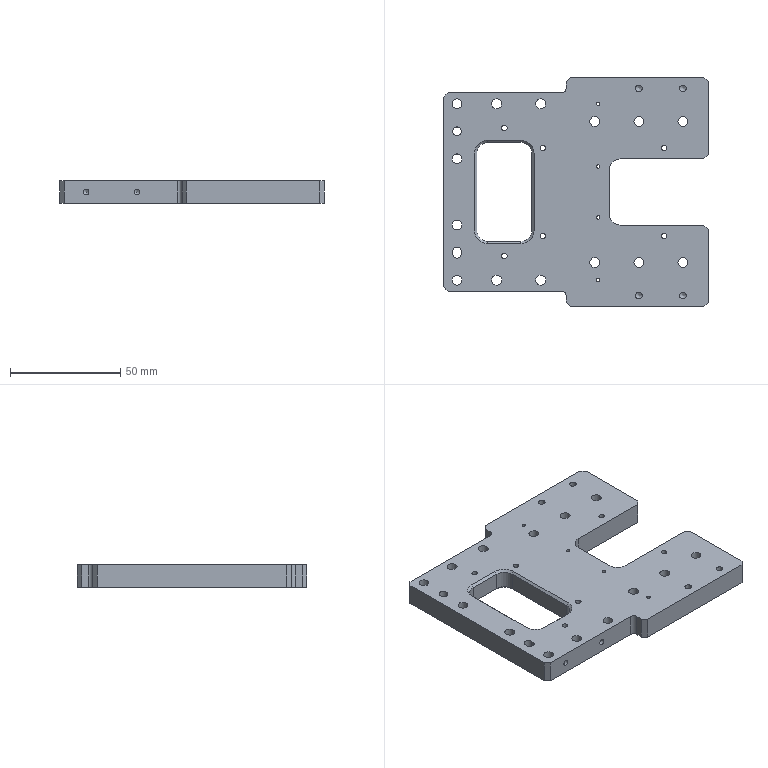CAM job | NX | 3-axis milling, drilling | part box 120 x 104 x 10 mm | stock box 125 x 109 x 12 mm
Tools:
number,name,description,diameter,corner_radius,flute_length,length,flutes
23,D2,平底铣刀-粗,2.0,0.0,50.0,75.0,2
3,D3,平底铣刀-粗,3.0,0.0,20.0,75.0,2
4,D4,平底铣刀-粗,4.0,0.0,25.0,75.0,2
9,D10,平底铣刀-粗,10.0,0.0,35.0,75.0,2
19,D2-J,平底铣刀-精,2.0,0.0,50.0,75.0,2
17,D3-J,平底铣刀-精,3.0,0.0,50.0,75.0,2
7,D6-J,平底铣刀-精,6.0,0.0,25.0,75.0,2
1,D80R0.8飞刀,圆鼻刀-粗,80.0,0.8,50.0,75.0,2
1,D80R0.8飞刀-J,圆鼻刀-精,80.0,0.8,50.0,75.0,2
2,D6倒角刀,倒角刀,6.0,0.0,3.0,25.0,2
18,M2X0.4,丝锥,1.6,0.0,35.0,50.0,2
20,M3X0.5,丝锥,2.5,0.0,35.0,50.0,2
24,D4铰刀,Drilling Tool,4.0,0.0,75.0,100.0,6
19,ZT1.6,钻头,1.6,0.0,35.0,50.0,2
12,ZT2.5,钻头,2.5,0.0,35.0,50.0,2
17,ZT2.8,钻头,2.8,0.0,35.0,50.0,2
11,ZT4.5,钻头,4.5,0.0,35.0,50.0,2
23,ZT3.9,Drilling Tool,3.9,0.0,35.0,50.0,2
Operations:
program,operation,operation_type,tool,method,geometry_group,spindle_rpm,surface_speed,feed_per_tooth,feed_cut,feed_plunge,cut_length_mm,path_length_mm,cut_time_min,machine_time_min
B,FLOORMILL_FACEROUGH_COPY,VolumeBased25DMillingOperation,D80R0.8飞刀,ZLEVEL_ROUGH-DEPTHK-STEPG,W-B,2800.0,703.696,0.5357,3000.0,100.0,1881.416,2062.298,0.6271,0.6452
B,FLOORMILL_FACEFINISH_COPY,VolumeBased25DMillingOperation,D80R0.8飞刀-J,SIDEMILL_FINISH-DEPTHK-STEPG,W-B,4000.0,1005.28,0.125,1000.0,100.0,469.767,505.767,0.4698,0.4734
B,SPOT-DEPTH1_2,Operation,D6倒角刀,NONE,W-B,8000.0,150.796,0.0312,500.0,90.0,52.2,664.384,0.1044,0.1656
B,BLINDCONE-FINISH3.0_PREDRILL,Operation,ZT2.8,NONE,W-B,3000.0,26.389,0.0133,80.0,90.0,27.205,231.466,0.3401,0.3605
B,HOLEMILL_ROUGHD2_1,CylinderMilling,D2,NONE,W-B,8000.0,50.266,0.0312,500.0,100.0,321.488,633.489,0.643,0.6742
B,C0.3_CLOSEDCONTOURCHAMFER6X45L_COPY_1,PlanarMilling,D6倒角刀,CLIMBFACE_CHAMFER-DEPTH0-STEPG,W-B,7000.0,131.0,0.1071,1500.0,100.0,141.508,177.508,0.0943,0.0979
B,DRILL_CHAMFER_4,Operation,D6倒角刀,METHOD,W-B,8000.0,150.796,0.0312,500.0,0.0,16.8,163.109,0.0336,0.0482
B,DRILL_CHAMFER_5,Operation,D6倒角刀,METHOD,W-B,8000.0,150.796,0.0312,500.0,0.0,28.5,299.124,0.057,0.0841
B,DRILL_CHAMFER_6,Operation,D6倒角刀,METHOD,W-B,8000.0,150.796,0.0312,500.0,0.0,19.2,221.895,0.0384,0.0587
B,DRILL_CHAMFER_7,Operation,D6倒角刀,METHOD,W-B,8000.0,150.796,0.0312,500.0,0.0,5.3,50.6,0.0106,0.0151
B,MILL_CHAMFER_2,PlanarMilling,D6倒角刀,METHOD,W-B,8000.0,150.796,0.0312,500.0,100.0,242.942,1102.162,0.4859,0.5718
B,C0.3_CLOSEDCONTOURCHAMFER6X45L_COPY,PlanarMilling,D6倒角刀,CLIMBFACE_CHAMFER-DEPTH0-STEPG,W-B,7000.0,131.0,0.1071,1500.0,100.0,563.445,753.143,0.3756,0.3946
B,FLOORMILL_CHAMFER_COPY_1,VolumeBased25DMillingOperation,D6倒角刀,CLIMBFACE_CHAMFER-DEPTH0-STEPG,W-B,6500.0,122.519,0.1154,1500.0,100.0,134.429,174.829,0.0896,0.0937
B,HOLEMILL_FINISHD2_1,CylinderMilling,D2-J,FINISH_STEPDEPTH_OFF,W-B,8000.0,50.266,0.0125,200.0,100.0,92.401,404.401,0.462,0.4932
A,TOPFACE,FaceMilling,D80R0.8飞刀,SIDEMILL_FINISH-DEPTHK-STEPG,W-A,4000.0,1005.31,0.125,1000.0,100.0,706.0,742.0,0.706,0.7096
A,CAVITYMILL_ROUGH-MEDIUM_COPY,CavityMilling,D10,ZLEVEL_ROUGH-DEPTHK-STEPG,W-A,8000.0,251.327,0.3125,5000.0,100.0,26282.6,26675.456,5.256,5.313
A,POCKET_ROUGH_1,VolumeBased25DMillingOperation,D10,METHOD,W-A,6000.0,188.0,0.25,4000.0,80.0,2183.925,2232.226,0.546,0.5508
A,SPOT-DEPTH1,Operation,D6倒角刀,NONE,W-A,8000.0,150.796,0.0312,500.0,90.0,46.8,678.022,0.0936,0.1567
A,THROUGHHOLE-M2_TAPDRILL,Operation,ZT1.6,NONE,W-A,3500.0,17.593,0.0043,30.0,90.0,61.923,246.902,2.064,2.083
A,THROUGHHOLE-M3_TAPDRILL,Operation,ZT2.5,NONE,W-A,3000.0,23.562,0.05,300.0,90.0,100.507,432.483,0.335,0.3682
A,THROUGHHOLE-FINISH4.0_PREDRILL,Operation,ZT3.9,NONE,W-A,3000.0,36.757,0.0417,250.0,90.0,30.252,156.012,0.121,0.1336
A,COUNTERBORE-DRILL_SEG0,Operation,ZT4.5,NONE,W-A,2800.0,39.584,0.0179,100.0,90.0,200.927,742.701,2.009,2.063
A,THROUGHSLOT_ROUGH_1,VolumeBased25DMillingOperation,D3,METHOD,W-A,6000.0,56.549,0.0667,800.0,100.0,358.896,407.695,0.4486,0.4535
A,HOLEMILL_ROUGHD4_1,CylinderMilling,D4,NONE,W-A,8000.0,100.531,0.075,1200.0,100.0,2981.396,3917.542,2.485,2.578
A,POCKET_SEMIFINISH_1,VolumeBased25DMillingOperation,D6-J,METHOD,W-A,6000.0,113.0,0.0833,1000.0,100.0,118.608,174.608,0.1186,0.1242
A,POCKET_FINISH_1,VolumeBased25DMillingOperation,D6-J,METHOD,W-A,6000.0,113.0,0.0833,1000.0,100.0,118.408,175.008,0.1184,0.1241
A,HOLEMILL_FINISHD4_1,CylinderMilling,D3-J,FINISH_STEPDEPTH_OFF,W-A,8000.0,100.531,0.0312,500.0,100.0,555.379,1491.525,1.111,1.204
A,PROFILE_SIDE,ZLevelMilling,D3-J,METHOD,W-A,9000.0,84.823,0.1389,2500.0,80.0,836.642,1029.483,0.3348,0.3541
A,SELECTBODYONLY,SurfaceContour,D6倒角刀,METHOD,W-A,8000.0,150.796,0.1875,3000.0,100.0,555.955,655.759,0.1853,0.1953
A,DRILL_CHAMFER_1,Operation,D6倒角刀,METHOD,W-A,8000.0,150.796,0.0312,500.0,0.0,16.8,163.109,0.0336,0.0482
A,DRILL_CHAMFER_2,Operation,D6倒角刀,METHOD,W-A,8000.0,150.796,0.0312,500.0,0.0,28.5,299.124,0.057,0.0841
A,DRILL_CHAMFER_3,Operation,D6倒角刀,METHOD,W-A,8000.0,150.796,0.0312,500.0,0.0,5.3,50.6,0.0106,0.0151
A,MILL_CHAMFER_1,PlanarMilling,D6倒角刀,NONE,W-A,8000.0,150.796,0.0312,500.0,100.0,475.55,1272.832,0.9511,1.031
A,FLOORMILL_CHAMFER_COPY,VolumeBased25DMillingOperation,D6倒角刀,CLIMBFACE_CHAMFER-DEPTH0-STEPG,W-A,6500.0,122.519,0.1154,1500.0,100.0,528.939,569.339,0.3526,0.3567
A,REAM,Operation,D4铰刀,METHOD,W-A,500.0,6.283,0.0167,50.0,0.0,12.0,64.0,0.24,0.2452
A,THROUGHHOLE-TAP_M2.0,Operation,M2X0.4,METHOD,W-A,1000.0,5.027,0.0002,0.4,90.0,56.0,235.057,140.0,140.018
A,THROUGHHOLE-TAP_M3,Operation,M3X0.5,METHOD,W-A,800.0,6.283,0.0003,0.5,90.0,84.0,399.471,168.0,168.031
A,SLOT_FINISH_1,VolumeBased25DMillingOperation,D3-J,METHOD,W-A,6000.0,113.0,0.0167,200.0,100.0,22.518,97.657,0.1126,0.1201
A,PROFILE_SEMIFINISH_2,VolumeBased25DMillingOperation,D6-J,METHOD,W-A,8000.0,251.327,0.0625,1000.0,100.0,545.526,604.726,0.5455,0.5514